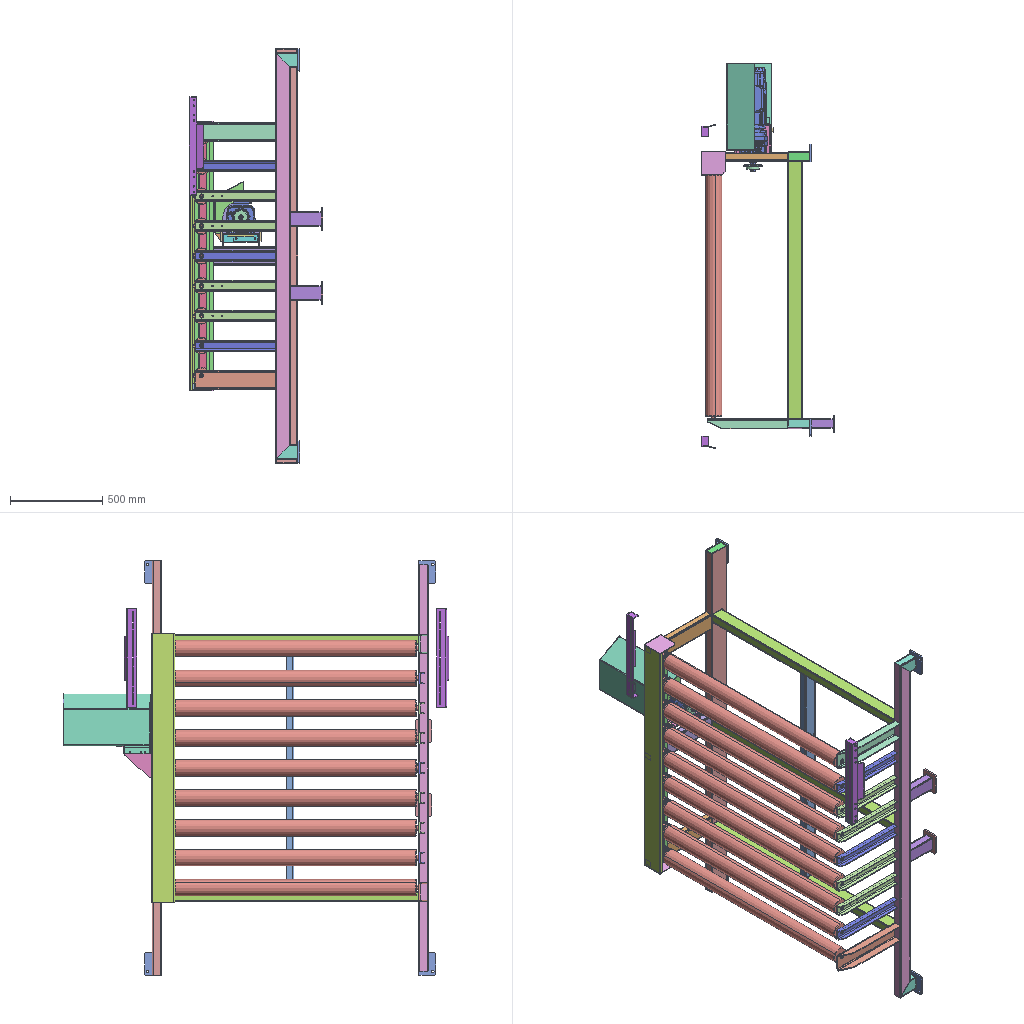Assembly | SolidWorks | 40 different items | 76 placed | box 724 x 2084 x 2240 mm
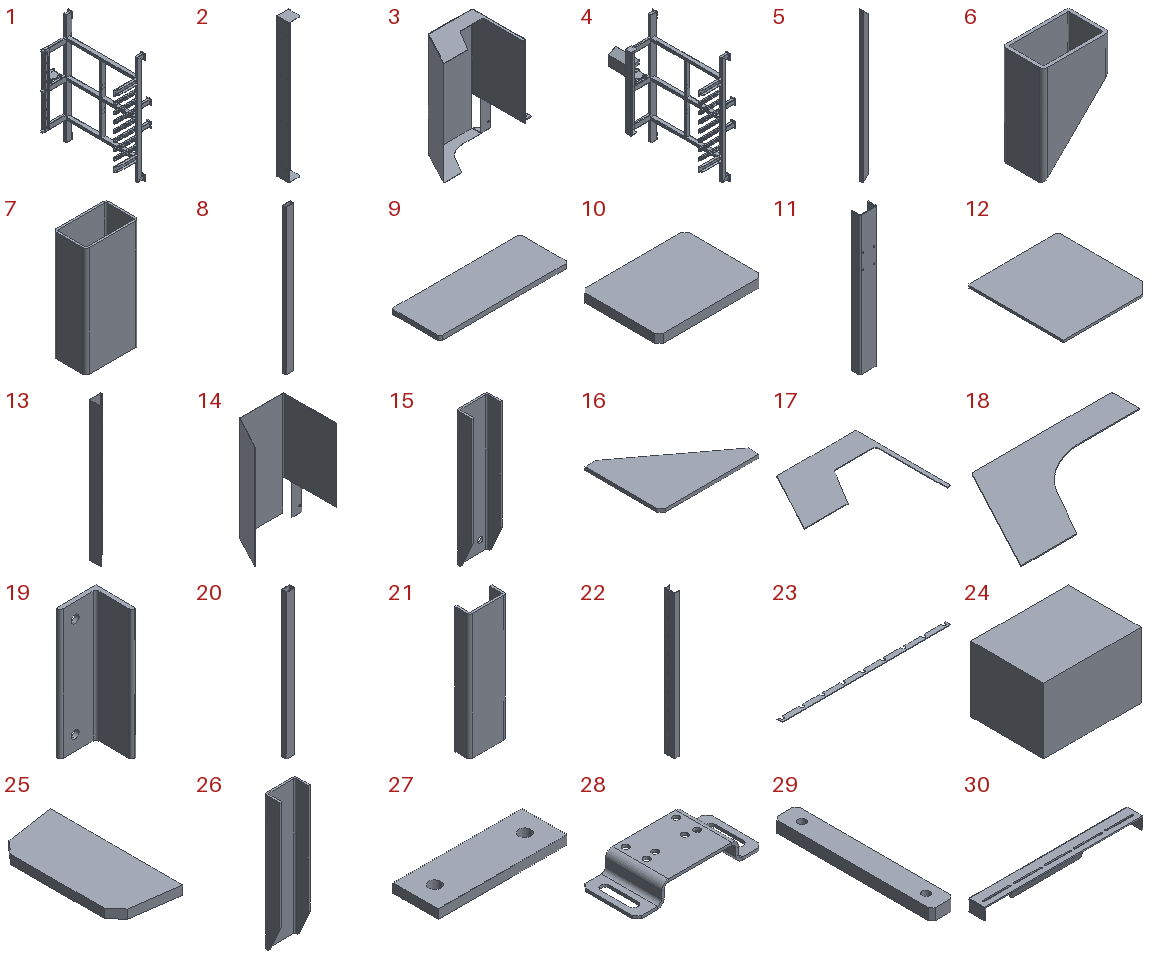Parts list (item | name | quantity | parent item | size | volume | features):
1 | (subassembly) | x1 | in 4 | 720.5 x 1683 x 2240 mm | 17379745 mm3 | features CompositeCurve 7
2 | (subassembly) | x1 | in 4 | 126 x 130 x 1460 mm | 1258975 mm3 | -
3 | (subassembly) | x1 | in 4 | 325 x 241.5 x 470 mm | 491131 mm3 | -
4 | (subassembly) | x1 | - | 723.5 x 2013 x 2240 mm | 19129851 mm3 | -
5 | - | x1 | in 1 | 80 x 50 x 2200 mm | 2025444 mm3 | features Extrusion 1, ICE 1, Shell 1
6 | - | x2 | in 1 | 80 x 50 x 120 mm | 76432 mm3 | features ICE 3, Extrusion 1, Shell 1
7 | - | x2 | in 1 | 80 x 50 x 166 mm | 120512 mm3 | features Extrusion 1, Fillet 1, Shell 1
8 | - | x1 | in 1 | 120 x 50 x 2240 mm | 2856892 mm3 | features Extrusion 1, Shell 1
9 | - | x2 | in 1 | 112 x 42 x 4 mm | 18802 mm3 | features Extrusion 1
10 | - | x2 | in 1 | 120 x 90 x 10 mm | 107500 mm3 | features Chamfer 1, Extrusion 1
11 | - | x2 | in 1 | 80 x 40 x 645 mm | 291778 mm3 | features Extrusion 1, ICE 1
12 | - | x2 | in 2 | 120 x 127 x 3 mm | 45371 mm3 | features Chamfer 2, Extrusion 1
13 | - | x1 | in 2 | 126 x 130 x 1460 mm | 1168234 mm3 | features Extrusion 1, ICE 1
14 | - | x1 | in 3 | 323.5 x 240 x 470 mm | 385016 mm3 | features ICE 4, Extrusion 1, MoveFace 1
15 | - | x1 | in 1 | 100 x 50 x 435 mm | 456835 mm3 | features ICE 2, Extrusion 1
16 | - | x2 | in 3 | 45 x 35 x 1.5 mm | 1460 mm3 | features Extrusion 1
17 | - | x1 | in 3 | 280 x 240 x 1.5 mm | 37497 mm3 | features Extrusion 1
18 | - | x1 | in 3 | 280 x 150 x 1.5 mm | 26833 mm3 | features Extrusion 1
19 | - | x1 | in 3 | 40 x 40 x 130 mm | 38867 mm3 | features Extrusion 1, Fillet 1, ICE 1
20 | - | x3 | in 1 | 80 x 50 x 1393 mm | 1330870 mm3 | features Extrusion 1, Shell 1
21 | - | x2 | in 1 | 100 x 40 x 337.5 mm | 331509 mm3 | features Extrusion 1
22 | - | x1 | in 1 | 50 x 100 x 1440 mm | 1898453 mm3 | features Extrusion 1, ICE 1
23 | - | x1 | in 1 | 1350 x 40 x 4 mm | 195775 mm3 | features Extrusion 1, Fillet 1, ICE 1
24 | - | x3 | in 1 | 40 x 30 x 27 mm | 32400 mm3 | features Extrusion 1
25 | - | x2 | in 1 | 40 x 88.903 x 6 mm | 19663 mm3 | features Extrusion 1
26 | - | x1 | in 1 | 100 x 50 x 435 mm | 456835 mm3 | features ICE 2, Extrusion 1
27 | - | x4 | in 1 | 86 x 30 x 6 mm | 14877 mm3 | features Extrusion 1, ICE 1
28 | - | x2 | - | 90 x 40 x 15 mm | 7851 mm3 | features EdgeFlange 2, ICE 2, Chamfer 1, FlatPattern 1, SMBaseFlange 1, SheetMetal 1
29 | - | x2 | - | 20 x 140 x 10 mm | 27094 mm3 | features 3DProfileFeature 1, Chamfer 1, Extrusion 1, HoleWzd 1
30 | - | x2 | - | 532 x 65.443 x 80 mm | 231503 mm3 | features ICE 3, EdgeFlange 2, Fillet 1, FlatPattern 1, SMBaseFlange 1, SheetMetal 1
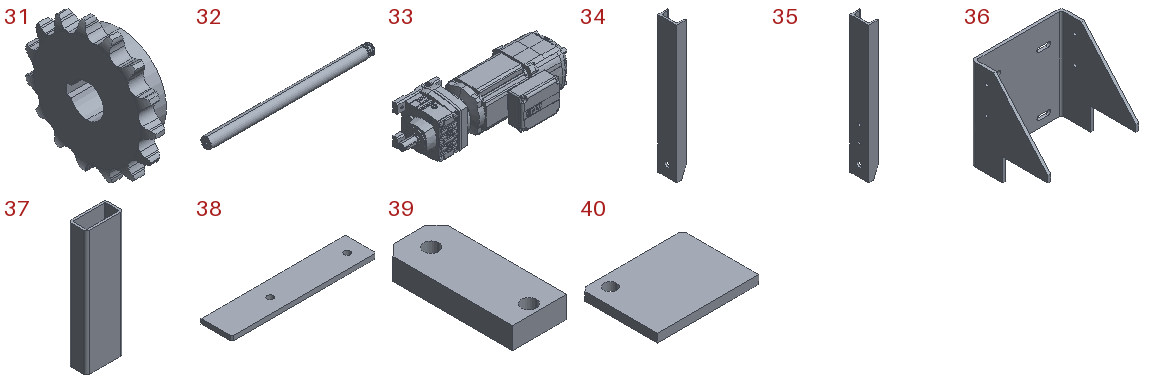31 | - | x1 | - | 25 x 98.203 x 98.722 mm | 107123 mm3 | features ICE 5, Chamfer 3, Cut 2, Revolution 2, CirPattern 1
32 | - | x9 | - | 1393 x 89 x 89 mm | 8327886 mm3 | features MoveFace 11, ICE 8, HoleWzd 3, BaseBody 1, Chamfer 1
33 | - | x1 | - | 564 x 218.4 x 161 mm | 9795428 mm3 | features BaseBody 1
34 | - | x3 | in 1 | 30 x 60 x 435 mm | 273006 mm3 | features ICE 2, Extrusion 1
35 | - | x4 | in 1 | 30 x 60 x 435 mm | 272325 mm3 | features ICE 3, Extrusion 1
36 | - | x1 | in 1 | 200 x 170 x 200 mm | 461581 mm3 | features ICE 3, Extrusion 1
37 | - | x1 | in 1 | 100 x 50 x 337.5 mm | 541517 mm3 | features Extrusion 1, Shell 1
38 | - | x1 | in 1 | 188 x 40 x 6 mm | 44493 mm3 | features Chamfer 1, Extrusion 1, ICE 1
39 | - | x2 | in 1 | 25 x 60 x 10 mm | 13980 mm3 | features Chamfer 1, Extrusion 1, ICE 1
40 | - | x4 | in 1 | 120 x 90 x 10 mm | 105983 mm3 | features Chamfer 1, Extrusion 1, ICE 1
Mates (type | each side: item.copy, entity, surface, feature):
In the top assembly
Coincident | 32.1 face plane QCH21-D89-W1182-t3-d20 | 32.2 face plane QCH21-D89-W1182-t3-d20
Coincident | 32.1 face plane QCH21-D89-W1182-t3-d20 | 32.3 face plane QCH21-D89-W1182-t3-d20
Coincident | 32.4 face plane QCH21-D89-W1182-t3-d20 | 32.3 face plane QCH21-D89-W1182-t3-d20
Coincident | 32.4 face plane QCH21-D89-W1182-t3-d20 | 32.5 face plane QCH21-D89-W1182-t3-d20
Coincident | 32.6 face plane QCH21-D89-W1182-t3-d20 | 32.5 face plane QCH21-D89-W1182-t3-d20
Coincident | 32.6 face plane QCH21-D89-W1182-t3-d20 | 32.7 face plane QCH21-D89-W1182-t3-d20
Coincident | 32.8 face plane QCH21-D89-W1182-t3-d20 | 32.9 face plane QCH21-D89-W1182-t3-d20
Coincident | 32.8 face plane QCH21-D89-W1182-t3-d20 | 32.7 face plane QCH21-D89-W1182-t3-d20
Concentric | 26.1 face cylinder Cut-Extrude1 | 32.7 face cylinder QCH21-D89-W1182-t3-d20
Concentric | 34.1 face cylinder Cut-Extrude1 | 32.8 face cylinder QCH21-D89-W1182-t3-d20
Concentric | 35.1 face cylinder Cut-Extrude1 | 32.9 face cylinder QCH21-D89-W1182-t3-d20
Concentric | 35.2 face cylinder Cut-Extrude1 | 32.6 face cylinder QCH21-D89-W1182-t3-d20
Concentric | 34.2 face cylinder Cut-Extrude1 | 32.5 face cylinder QCH21-D89-W1182-t3-d20
Concentric | 35.3 face cylinder Cut-Extrude1 | 32.4 face cylinder QCH21-D89-W1182-t3-d20
Concentric | 35.4 face cylinder Cut-Extrude1 | 32.3 face cylinder QCH21-D89-W1182-t3-d20
Concentric | 34.3 face cylinder Cut-Extrude1 | 32.1 face cylinder QCH21-D89-W1182-t3-d20
Concentric | 15.1 face cylinder Cut-Extrude1 | 32.2 face cylinder QCH21-D89-W1182-t3-d20
Coincident | 15.1 face plane Boss-Extrude1 | 32.2 face plane Boss-Extrude2
Parallel | 34.1 face plane Boss-Extrude1 | 32.8 face plane QCH21-D89-W1182-t3-d20
Parallel | 35.1 face plane Boss-Extrude1 | 32.9 face plane QCH21-D89-W1182-t3-d20
Parallel | 35.2 face plane Boss-Extrude1 | 32.6 face plane QCH21-D89-W1182-t3-d20
Parallel | 34.2 face plane Boss-Extrude1 | 32.5 face plane QCH21-D89-W1182-t3-d20
Parallel | 35.4 face plane Boss-Extrude1 | 32.3 face plane QCH21-D89-W1182-t3-d20
Parallel | 35.3 face plane Boss-Extrude1 | 32.4 face plane QCH21-D89-W1182-t3-d20
Parallel | 34.3 face plane Boss-Extrude1 | 32.1 face plane QCH21-D89-W1182-t3-d20
Parallel | 26.1 face plane Boss-Extrude1 | 32.7 face plane QCH21-D89-W1182-t3-d20
Coincident | 29.1 face plane Boss-Extrude1 | 29.2 face plane Boss-Extrude1
Coincident | 36.1 face plane Boss-Extrude2 | 29.2 face plane Boss-Extrude1
Slot | 29.2 face cylinder M8 Tapped Hole1 | 36.1 face plane Cut-Extrude3
Slot | 36.1 face plane Cut-Extrude3 | 29.2 face cylinder M8 Tapped Hole1
Slot | 29.1 face cylinder M8 Tapped Hole1 | 36.1 face plane Cut-Extrude3 | 2 times
Coincident | 28.1 face plane Edge-Flange2 | 30.1 face plane Base-Flange1
Slot | 28.1 face plane Cut-Extrude1 | 30.1 face plane Cut-Extrude2
Slot | 30.1 face plane Cut-Extrude2 | 28.1 face cylinder Cut-Extrude1
Coincident | 28.1 face plane Edge-Flange1 | 30.1 edge
Parallel | 14.1 face plane Boss-Extrude1 | 30.1 face plane Base-Flange1
Parallel | 12.1 face plane Boss-Extrude1 | 30.1 face plane Edge-Flange2
Slot | 28.2 face cylinder Cut-Extrude1 | 30.2 face plane Cut-Extrude2
Slot | 30.2 face plane Cut-Extrude2 | 28.2 face plane Cut-Extrude1
Coincident | 30.2 face plane Base-Flange1 | 28.2 face plane Edge-Flange2 | 2 times
Lock | 12.1 select_type:0 | 30.1 select_type:0
Coincident | 30.1 face plane Edge-Flange2 | 30.2 face plane Edge-Flange2
Coincident | 30.1 face plane Base-Flange1 | 30.2 face plane Base-Flange1
Coincident | 36.1 face plane Boss-Extrude2 | 33.1 face plane Input1
Concentric | 29.2 face cylinder M8 Tapped Hole1 | 33.1 face cylinder Input1 | 2 times
Concentric | 31.1 face cylinder Cut-Extrude5 | 33.1 face cylinder Input1
Parallel | 31.1 face plane Cut-Extrude6 | 33.1 face plane Input1
In subassembly 4
Width | 12.2 face plane Boss-Extrude1 | 12.3 face plane Boss-Extrude1 | 25.1 face plane Boss-Extrude1 | 25.2 face plane Boss-Extrude1
Concentric | 27.1 face cylinder Cut-Extrude1 | 13.1 face cylinder Cut-Extrude1
Coincident | 27.2 face plane Boss-Extrude1 | 13.1 face plane Boss-Extrude1
Concentric | 38.1 face cylinder Cut-Extrude1 | 19.1 face cylinder Cut-Extrude1 | 2 times
Coincident | 38.1 face plane Boss-Extrude1 | 19.1 face plane Boss-Extrude1
In subassembly 3
Coincident | 14.2 face plane Boss-Extrude3 | 16.1 face plane Boss-Extrude1 | 2 times
Coincident | 14.2 face plane Boss-Extrude1 | 16.2 face plane Boss-Extrude1
Coincident | 14.2 face plane Boss-Extrude3 | 16.2 face plane Boss-Extrude1
Coincident | 14.2 edge | 16.2 face plane Boss-Extrude1
Coincident | 16.1 face plane Boss-Extrude1 | 16.2 face plane Boss-Extrude1
Coincident | 14.2 face plane Boss-Extrude1 | 17.1 face plane Boss-Extrude1 | 3 times
Coincident | 14.2 face plane Boss-Extrude1 | 18.1 face plane Boss-Extrude1 | 3 times
Coincident | 16.1 face plane Boss-Extrude1 | 19.2 face plane Boss-Extrude1
Coincident | 14.2 face plane Boss-Extrude1 | 19.2 face plane Boss-Extrude1
DistanceDim | 19.2 face plane Boss-Extrude1 | 14.2 face plane Boss-Extrude1
In subassembly 2
Coincident | 13.2 face plane Boss-Extrude1 | 12.4 face plane Boss-Extrude1 | 3 times
Coincident | 12.5 face plane Boss-Extrude1 | 12.4 face plane Boss-Extrude1 | 2 times
Coincident | 13.2 face plane Boss-Extrude1 | 12.5 face plane Boss-Extrude1
In subassembly 1
Coincident | 8.1 face plane Boss-Extrude1 | 40.1 face plane Boss-Extrude1 | 3 times
Coincident | 8.1 face plane Boss-Extrude1 | 40.2 face plane Boss-Extrude1 | 2 times
Coincident | 8.1 face plane Boss-Extrude1 | 20.1 face plane Boss-Extrude1
Coincident | 8.1 face plane Boss-Extrude1 | 20.2 face plane Boss-Extrude1 | 2 times
Coincident | 20.1 face plane Boss-Extrude1 | 20.2 face plane Boss-Extrude1
Coincident | 20.3 face plane Boss-Extrude1 | 20.2 face plane Boss-Extrude1 | 2 times
DistanceDim | 20.1 face plane Boss-Extrude1 | 20.3 face plane Boss-Extrude1
DistanceDim | 20.3 face plane Boss-Extrude1 | 20.2 face plane Boss-Extrude1
DistanceDim | 20.1 face plane Boss-Extrude1 | 8.1 face plane Boss-Extrude1
Coincident | 20.3 face plane Boss-Extrude1 | 5.1 face plane Boss-Extrude1
Coincident | 20.1 face plane Boss-Extrude1 | 5.1 face plane Boss-Extrude1
Coincident | 5.1 face plane Cut-Extrude2 | 6.1 face plane Cut-Extrude2
Coincident | 5.1 face plane Boss-Extrude1 | 6.1 face plane Boss-Extrude1
Coincident | 5.1 edge | 6.1 edge
Coincident | 5.1 face plane Boss-Extrude1 | 6.2 face plane Boss-Extrude1
Coincident | 5.1 edge | 6.2 edge
Coincident | 5.1 face plane Cut-Extrude2 | 6.2 face plane Cut-Extrude2
Width | 6.2 face plane Boss-Extrude1 | 6.1 face plane Boss-Extrude1 | 20.1 face plane Boss-Extrude1 | 20.2 face plane Boss-Extrude1
Coincident | 8.1 face plane Boss-Extrude1 | 21.1 face plane Boss-Extrude2
Coincident | 21.1 face plane Boss-Extrude2 | 21.2 face plane Boss-Extrude2 | 2 times
Coincident | 8.1 face plane Boss-Extrude1 | 21.2 face plane Boss-Extrude2
Coincident | 20.1 face plane Boss-Extrude1 | 21.2 face plane Boss-Extrude2
Coincident | 20.2 face plane Boss-Extrude1 | 21.1 face plane Boss-Extrude2
Coincident | 8.1 face plane Boss-Extrude1 | 37.1 face plane Boss-Extrude2 | 2 times
Width | 37.1 face plane Boss-Extrude2 | 37.1 face plane Boss-Extrude2 | 20.3 face plane Boss-Extrude1 | 20.3 face plane Boss-Extrude1
Coincident | 21.2 face plane Boss-Extrude2 | 22.1 face plane Boss-Extrude1 | 3 times
Coincident | 22.1 face plane Boss-Extrude1 | 23.1 face plane Boss-Extrude1
Concentric | 22.1 edge | 23.1 edge | 2 times
Coincident | 22.1 face plane Boss-Extrude1 | 24.1 face plane Boss-Extrude1 | 2 times
DistanceDim | 24.1 face plane Boss-Extrude1 | 22.1 face plane Boss-Extrude1
Coincident | 24.1 face plane Boss-Extrude1 | 24.2 face plane Boss-Extrude1 | 2 times
Coincident | 24.1 face plane Boss-Extrude1 | 24.3 face plane Boss-Extrude1 | 2 times
DistanceDim | 24.2 face plane Boss-Extrude1 | 24.1 edge
DistanceDim | 24.3 face plane Boss-Extrude1 | 24.2 face plane Boss-Extrude1
Coincident | 22.1 face plane Boss-Extrude1 | 25.3 face plane Boss-Extrude1 | 3 times
Coincident | 25.3 face plane Boss-Extrude1 | 25.4 face plane Boss-Extrude1
Coincident | 22.1 face plane Boss-Extrude1 | 25.4 face plane Boss-Extrude1 | 2 times
Coincident | 37.1 face plane Boss-Extrude2 | 27.3 face plane Boss-Extrude1
Width | 27.3 face plane Boss-Extrude1 | 27.3 face plane Boss-Extrude1 | 22.1 face plane Boss-Extrude1 | 22.1 face plane Boss-Extrude1
Coincident | 27.4 face plane Boss-Extrude1 | 27.5 face plane Boss-Extrude1 | 2 times
Coincident | 27.6 face plane Boss-Extrude1 | 27.4 face plane Boss-Extrude1 | 2 times
Parallel | 27.6 face plane Boss-Extrude1 | 27.3 face plane Boss-Extrude1
Coincident | 27.3 face plane Boss-Extrude1 | 27.4 face plane Boss-Extrude1 | 2 times
Coincident | 5.1 face plane Boss-Extrude1 | 15.2 face plane Boss-Extrude1 | 2 times
Coincident | 5.1 face plane Boss-Extrude1 | 26.2 face plane Boss-Extrude1 | 2 times
Coincident | 5.1 face plane Boss-Extrude1 | 34.4 face plane Boss-Extrude1 | 2 times
Coincident | 34.4 face plane Boss-Extrude1 | 34.5 face plane Boss-Extrude1
Coincident | 34.6 face plane Boss-Extrude1 | 34.5 face plane Boss-Extrude1
Coincident | 5.1 face plane Boss-Extrude1 | 35.5 face plane Boss-Extrude1 | 2 times
Coincident | 35.5 face plane Boss-Extrude1 | 35.6 face plane Boss-Extrude1
Coincident | 37.1 face plane Boss-Extrude2 | 36.2 face plane Cut-Extrude1 | 2 times
DistanceDim | 36.2 face plane Boss-Extrude2 | 22.1 face plane Boss-Extrude1
Coincident | 36.2 face plane Boss-Extrude2 | 38.2 face plane Boss-Extrude1 | 3 times
Coincident | 36.2 face plane Boss-Extrude2 | 39.1 face plane Boss-Extrude1
Concentric | 36.2 edge | 39.1 edge
Parallel | 36.2 face plane Boss-Extrude2 | 39.1 face plane Boss-Extrude1
Coincident | 36.2 face plane Boss-Extrude2 | 39.2 face plane Boss-Extrude1
Coincident | 39.1 face plane Boss-Extrude1 | 39.2 face plane Boss-Extrude1
Coincident | 7.1 face plane Boss-Extrude1 | 7.2 face plane Boss-Extrude1
Coincident | 5.1 face plane Boss-Extrude1 | 7.1 face plane Boss-Extrude1 | 2 times
Coincident | 5.1 face plane Boss-Extrude1 | 7.2 face plane Boss-Extrude1
DistanceDim | 7.2 face plane Boss-Extrude1 | 6.1 face plane Boss-Extrude1
DistanceDim | 7.1 face plane Boss-Extrude1 | 7.2 face plane Boss-Extrude1
Coincident | 8.1 face plane Boss-Extrude1 | 9.1 face plane Boss-Extrude1
Coincident | 8.1 face plane Shell1 | 9.1 face plane Boss-Extrude1 | 2 times
Coincident | 8.1 face plane Boss-Extrude1 | 9.2 face plane Boss-Extrude1
Coincident | 8.1 face plane Shell1 | 9.2 face plane Boss-Extrude1 | 2 times
Width | 10.1 face plane Boss-Extrude1 | 10.1 face plane Boss-Extrude1 | 5.1 face plane Boss-Extrude1 | 5.1 face plane Boss-Extrude1
Coincident | 10.1 face plane Boss-Extrude1 | 10.2 face plane Boss-Extrude1
Coincident | 7.2 face plane Boss-Extrude1 | 10.1 face plane Boss-Extrude1
Coincident | 7.1 face plane Boss-Extrude1 | 10.2 face plane Boss-Extrude1
Width | 7.1 face plane Boss-Extrude1 | 7.1 face plane Boss-Extrude1 | 10.2 face plane Boss-Extrude1 | 10.2 face plane Boss-Extrude1
Width | 7.2 face plane Boss-Extrude1 | 7.2 face plane Boss-Extrude1 | 10.1 face plane Boss-Extrude1 | 10.1 face plane Boss-Extrude1
Coincident | 40.1 face plane Boss-Extrude1 | 40.3 face plane Boss-Extrude1 | 2 times
Coincident | 5.1 face plane Boss-Extrude1 | 40.3 face plane Boss-Extrude1
Coincident | 5.1 face plane Boss-Extrude1 | 40.4 face plane Boss-Extrude1
Coincident | 6.2 face plane Cut-Extrude3 | 40.4 face plane Boss-Extrude1
Coincident | 20.3 face plane Boss-Extrude1 | 11.1 face plane Boss-Extrude1 | 2 times
Coincident | 11.1 face plane Boss-Extrude1 | 11.2 face plane Boss-Extrude1 | 2 times
Coincident | 20.1 face plane Boss-Extrude1 | 11.2 face plane Boss-Extrude1
Width | 11.2 face plane Boss-Extrude1 | 11.2 face plane Boss-Extrude1 | 8.1 face plane Boss-Extrude1 | 5.1 face plane Boss-Extrude1
DistanceDim | 27.6 face cylinder Cut-Extrude1 | 27.5 face cylinder Cut-Extrude1
DistanceDim | 27.5 face cylinder Cut-Extrude1 | 27.4 face cylinder Cut-Extrude1
DistanceDim | 27.4 face cylinder Cut-Extrude1 | 27.3 face cylinder Cut-Extrude1
Width | 27.6 face plane Boss-Extrude1 | 27.3 face plane Boss-Extrude1 | 25.3 face plane Boss-Extrude1 | 25.4 face plane Boss-Extrude1
Coincident | 5.1 face plane Boss-Extrude1 | 34.6 face plane Boss-Extrude1
Coincident | 5.1 face plane Boss-Extrude1 | 35.6 face plane Boss-Extrude1
Coincident | 5.1 face plane Boss-Extrude1 | 34.5 face plane Boss-Extrude1
Coincident | 5.1 face plane Boss-Extrude1 | 35.7 face plane Boss-Extrude1
Coincident | 5.1 face plane Boss-Extrude1 | 35.8 face plane Boss-Extrude1
Coincident | 34.4 face plane Boss-Extrude1 | 35.7 face plane Boss-Extrude1
Coincident | 34.4 face plane Boss-Extrude1 | 35.8 face plane Boss-Extrude1
DistanceDim | 35.7 face cylinder Cut-Extrude1 | 34.4 face cylinder Cut-Extrude1
DistanceDim | 35.8 face cylinder Cut-Extrude1 | 35.7 face cylinder Cut-Extrude1
DistanceDim | 34.5 face cylinder Cut-Extrude1 | 35.8 face cylinder Cut-Extrude1
DistanceDim | 35.5 face cylinder Cut-Extrude1 | 34.5 face cylinder Cut-Extrude1
Coincident | 20.1 face plane Boss-Extrude1 | 26.2 face plane Boss-Extrude1
DistanceDim | 26.2 face cylinder Cut-Extrude1 | 34.4 face cylinder Cut-Extrude1
Coincident | 20.2 face plane Boss-Extrude1 | 15.2 face plane Boss-Extrude1
DistanceDim | 35.5 face cylinder Cut-Extrude1 | 35.6 face cylinder Cut-Extrude1
DistanceDim | 35.6 face cylinder Cut-Extrude1 | 34.6 face cylinder Cut-Extrude1
Coincident | 40.2 face plane Boss-Extrude1 | 9.1 face plane Boss-Extrude1
Coincident | 40.2 face plane Boss-Extrude1 | 40.4 face plane Boss-Extrude1